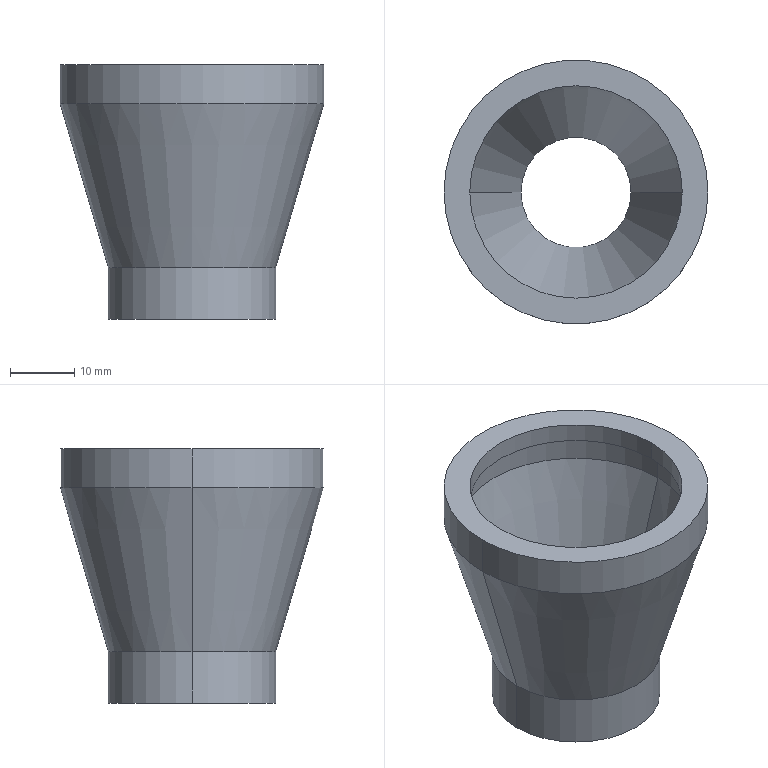Part | NX | features BREP 1 | 1 solid | 15 faces | box 41 x 41 x 39.5 mm | volume 9433 mm3 | cylinder 8 | cone 4 | plane 3 | commonest cylinder face diameters 26 x2 33 x2 36 x2 41 x2
STEP:
#1=CARTESIAN_POINT('',(13.,0.,-51.5));
#2=VERTEX_POINT('',#1);
#3=CARTESIAN_POINT('',(-13.,0.,-51.5));
#4=VERTEX_POINT('',#3);
#5=CARTESIAN_POINT('',(0.,0.,-51.5));
#6=DIRECTION('',(0.,0.,1.));
#7=DIRECTION('',(1.,0.,0.));
#8=AXIS2_PLACEMENT_3D('',#5,#6,#7);
#9=CIRCLE('',#8,13.);
#10=EDGE_CURVE('',#2,#4,#9,.T.);
#11=ORIENTED_EDGE('',*,*,#10,.T.);
#12=CARTESIAN_POINT('',(-20.5,0.,-26.));
#13=VERTEX_POINT('',#12);
#14=CARTESIAN_POINT('',(-20.5,0.,-26.));
#15=DIRECTION('',(-0.2822,0.,0.9594));
#16=VECTOR('',#15,1000.);
#17=LINE('',#14,#16);
#18=EDGE_CURVE('',#13,#4,#17,.F.);
#19=ORIENTED_EDGE('',*,*,#18,.F.);
#20=CARTESIAN_POINT('',(20.5,0.,-26.));
#21=VERTEX_POINT('',#20);
#22=CARTESIAN_POINT('',(0.,0.,-26.));
#23=DIRECTION('',(0.,0.,-1.));
#24=DIRECTION('',(1.,0.,0.));
#25=AXIS2_PLACEMENT_3D('',#22,#23,#24);
#26=CIRCLE('',#25,20.5);
#27=EDGE_CURVE('',#13,#21,#26,.T.);
#28=ORIENTED_EDGE('',*,*,#27,.T.);
#29=CARTESIAN_POINT('',(20.5,0.,-26.));
#30=DIRECTION('',(0.2822,0.,0.9594));
#31=VECTOR('',#30,1000.);
#32=LINE('',#29,#31);
#33=EDGE_CURVE('',#21,#2,#32,.F.);
#34=ORIENTED_EDGE('',*,*,#33,.T.);
#35=EDGE_LOOP('',(#11,#19,#28,#34));
#36=FACE_BOUND('',#35,.T.);
#37=CARTESIAN_POINT('',(0.,0.,-26.));
#38=DIRECTION('',(0.,0.,1.));
#39=DIRECTION('',(1.,0.,0.));
#40=AXIS2_PLACEMENT_3D('',#37,#38,#39);
#41=CONICAL_SURFACE('',#40,20.5,0.2861);
#42=ADVANCED_FACE('',(#36),#41,.T.);
#43=CARTESIAN_POINT('',(-20.5,0.,-20.));
#44=VERTEX_POINT('',#43);
#45=CARTESIAN_POINT('',(20.5,0.,-20.));
#46=VERTEX_POINT('',#45);
#47=CARTESIAN_POINT('',(0.,0.,-20.));
#48=DIRECTION('',(0.,0.,-1.));
#49=DIRECTION('',(-1.,0.,0.));
#50=AXIS2_PLACEMENT_3D('',#47,#48,#49);
#51=CIRCLE('',#50,20.5);
#52=EDGE_CURVE('',#44,#46,#51,.T.);
#53=ORIENTED_EDGE('',*,*,#52,.T.);
#54=CARTESIAN_POINT('',(20.5,0.,-23.));
#55=DIRECTION('',(0.,0.,-1.));
#56=VECTOR('',#55,1000.);
#57=LINE('',#54,#56);
#58=EDGE_CURVE('',#46,#21,#57,.T.);
#59=ORIENTED_EDGE('',*,*,#58,.T.);
#60=ORIENTED_EDGE('',*,*,#27,.F.);
#61=CARTESIAN_POINT('',(-20.5,0.,-23.));
#62=DIRECTION('',(0.,0.,-1.));
#63=VECTOR('',#62,1000.);
#64=LINE('',#61,#63);
#65=EDGE_CURVE('',#44,#13,#64,.T.);
#66=ORIENTED_EDGE('',*,*,#65,.F.);
#67=EDGE_LOOP('',(#53,#59,#60,#66));
#68=FACE_BOUND('',#67,.T.);
#69=CARTESIAN_POINT('',(0.,0.,-23.));
#70=DIRECTION('',(0.,0.,-1.));
#71=DIRECTION('',(-1.,0.,0.));
#72=AXIS2_PLACEMENT_3D('',#69,#70,#71);
#73=CYLINDRICAL_SURFACE('',#72,20.5);
#74=ADVANCED_FACE('',(#68),#73,.T.);
#75=ORIENTED_EDGE('',*,*,#10,.F.);
#76=CARTESIAN_POINT('',(13.,0.,-59.5));
#77=VERTEX_POINT('',#76);
#78=CARTESIAN_POINT('',(13.,0.,-55.5));
#79=DIRECTION('',(0.,0.,-1.));
#80=VECTOR('',#79,1000.);
#81=LINE('',#78,#80);
#82=EDGE_CURVE('',#2,#77,#81,.T.);
#83=ORIENTED_EDGE('',*,*,#82,.T.);
#84=CARTESIAN_POINT('',(-13.,0.,-59.5));
#85=VERTEX_POINT('',#84);
#86=CARTESIAN_POINT('',(0.,0.,-59.5));
#87=DIRECTION('',(0.,0.,1.));
#88=DIRECTION('',(-1.,0.,0.));
#89=AXIS2_PLACEMENT_3D('',#86,#87,#88);
#90=CIRCLE('',#89,13.);
#91=EDGE_CURVE('',#77,#85,#90,.T.);
#92=ORIENTED_EDGE('',*,*,#91,.T.);
#93=CARTESIAN_POINT('',(-13.,0.,-55.5));
#94=DIRECTION('',(0.,0.,-1.));
#95=VECTOR('',#94,1000.);
#96=LINE('',#93,#95);
#97=EDGE_CURVE('',#4,#85,#96,.T.);
#98=ORIENTED_EDGE('',*,*,#97,.F.);
#99=EDGE_LOOP('',(#75,#83,#92,#98));
#100=FACE_BOUND('',#99,.T.);
#101=CARTESIAN_POINT('',(0.,0.,-55.5));
#102=DIRECTION('',(0.,0.,-1.));
#103=DIRECTION('',(-1.,0.,0.));
#104=AXIS2_PLACEMENT_3D('',#101,#102,#103);
#105=CYLINDRICAL_SURFACE('',#104,13.);
#106=ADVANCED_FACE('',(#100),#105,.T.);
#107=CARTESIAN_POINT('',(16.5,0.,-20.));
#108=VERTEX_POINT('',#107);
#109=CARTESIAN_POINT('',(-16.5,0.,-20.));
#110=VERTEX_POINT('',#109);
#111=CARTESIAN_POINT('',(0.,0.,-20.));
#112=DIRECTION('',(0.,0.,-1.));
#113=DIRECTION('',(-1.,0.,0.));
#114=AXIS2_PLACEMENT_3D('',#111,#112,#113);
#115=CIRCLE('',#114,16.5);
#116=EDGE_CURVE('',#108,#110,#115,.T.);
#117=ORIENTED_EDGE('',*,*,#116,.F.);
#118=CARTESIAN_POINT('',(16.5,0.,-22.99));
#119=VERTEX_POINT('',#118);
#120=CARTESIAN_POINT('',(16.5,0.,-21.495));
#121=DIRECTION('',(0.,0.,-1.));
#122=VECTOR('',#121,1000.);
#123=LINE('',#120,#122);
#124=EDGE_CURVE('',#108,#119,#123,.T.);
#125=ORIENTED_EDGE('',*,*,#124,.T.);
#126=CARTESIAN_POINT('',(-16.5,0.,-22.99));
#127=VERTEX_POINT('',#126);
#128=CARTESIAN_POINT('',(0.,0.,-22.99));
#129=DIRECTION('',(0.,0.,1.));
#130=DIRECTION('',(-1.,0.,0.));
#131=AXIS2_PLACEMENT_3D('',#128,#129,#130);
#132=CIRCLE('',#131,16.5);
#133=EDGE_CURVE('',#127,#119,#132,.T.);
#134=ORIENTED_EDGE('',*,*,#133,.F.);
#135=CARTESIAN_POINT('',(-16.5,0.,-21.495));
#136=DIRECTION('',(0.,0.,-1.));
#137=VECTOR('',#136,1000.);
#138=LINE('',#135,#137);
#139=EDGE_CURVE('',#110,#127,#138,.T.);
#140=ORIENTED_EDGE('',*,*,#139,.F.);
#141=EDGE_LOOP('',(#117,#125,#134,#140));
#142=FACE_BOUND('',#141,.T.);
#143=CARTESIAN_POINT('',(0.,0.,-21.495));
#144=DIRECTION('',(0.,0.,-1.));
#145=DIRECTION('',(-1.,0.,0.));
#146=AXIS2_PLACEMENT_3D('',#143,#144,#145);
#147=CYLINDRICAL_SURFACE('',#146,16.5);
#148=ADVANCED_FACE('',(#142),#147,.F.);
#149=CARTESIAN_POINT('',(-8.562,0.,-59.5));
#150=VERTEX_POINT('',#149);
#151=CARTESIAN_POINT('',(8.562,0.,-59.5));
#152=VERTEX_POINT('',#151);
#153=CARTESIAN_POINT('',(0.,0.,-59.5));
#154=DIRECTION('',(0.,0.,1.));
#155=DIRECTION('',(1.,0.,0.));
#156=AXIS2_PLACEMENT_3D('',#153,#154,#155);
#157=CIRCLE('',#156,8.562);
#158=EDGE_CURVE('',#150,#152,#157,.T.);
#159=ORIENTED_EDGE('',*,*,#158,.F.);
#160=CARTESIAN_POINT('',(-18.,0.,-27.412));
#161=VERTEX_POINT('',#160);
#162=CARTESIAN_POINT('',(-18.,0.,-27.412));
#163=DIRECTION('',(-0.2822,0.,0.9594));
#164=VECTOR('',#163,1000.);
#165=LINE('',#162,#164);
#166=EDGE_CURVE('',#161,#150,#165,.F.);
#167=ORIENTED_EDGE('',*,*,#166,.F.);
#168=CARTESIAN_POINT('',(18.,0.,-27.412));
#169=VERTEX_POINT('',#168);
#170=CARTESIAN_POINT('',(0.,0.,-27.412));
#171=DIRECTION('',(0.,0.,-1.));
#172=DIRECTION('',(1.,0.,0.));
#173=AXIS2_PLACEMENT_3D('',#170,#171,#172);
#174=CIRCLE('',#173,18.);
#175=EDGE_CURVE('',#169,#161,#174,.T.);
#176=ORIENTED_EDGE('',*,*,#175,.F.);
#177=CARTESIAN_POINT('',(18.,0.,-27.412));
#178=DIRECTION('',(0.2822,0.,0.9594));
#179=VECTOR('',#178,1000.);
#180=LINE('',#177,#179);
#181=EDGE_CURVE('',#169,#152,#180,.F.);
#182=ORIENTED_EDGE('',*,*,#181,.T.);
#183=EDGE_LOOP('',(#159,#167,#176,#182));
#184=FACE_BOUND('',#183,.T.);
#185=CARTESIAN_POINT('',(0.,0.,-27.412));
#186=DIRECTION('',(0.,0.,1.));
#187=DIRECTION('',(1.,0.,0.));
#188=AXIS2_PLACEMENT_3D('',#185,#186,#187);
#189=CONICAL_SURFACE('',#188,18.,0.2861);
#190=ADVANCED_FACE('',(#184),#189,.F.);
#191=CARTESIAN_POINT('',(18.,0.,-22.99));
#192=VERTEX_POINT('',#191);
#193=CARTESIAN_POINT('',(-18.,0.,-22.99));
#194=VERTEX_POINT('',#193);
#195=CARTESIAN_POINT('',(0.,0.,-22.99));
#196=DIRECTION('',(0.,0.,-1.));
#197=DIRECTION('',(-1.,0.,0.));
#198=AXIS2_PLACEMENT_3D('',#195,#196,#197);
#199=CIRCLE('',#198,18.);
#200=EDGE_CURVE('',#192,#194,#199,.T.);
#201=ORIENTED_EDGE('',*,*,#200,.F.);
#202=CARTESIAN_POINT('',(18.,0.,-25.201));
#203=DIRECTION('',(0.,0.,-1.));
#204=VECTOR('',#203,1000.);
#205=LINE('',#202,#204);
#206=EDGE_CURVE('',#192,#169,#205,.T.);
#207=ORIENTED_EDGE('',*,*,#206,.T.);
#208=ORIENTED_EDGE('',*,*,#175,.T.);
#209=CARTESIAN_POINT('',(-18.,0.,-25.201));
#210=DIRECTION('',(0.,0.,-1.));
#211=VECTOR('',#210,1000.);
#212=LINE('',#209,#211);
#213=EDGE_CURVE('',#194,#161,#212,.T.);
#214=ORIENTED_EDGE('',*,*,#213,.F.);
#215=EDGE_LOOP('',(#201,#207,#208,#214));
#216=FACE_BOUND('',#215,.T.);
#217=CARTESIAN_POINT('',(0.,0.,-25.201));
#218=DIRECTION('',(0.,0.,-1.));
#219=DIRECTION('',(-1.,0.,0.));
#220=AXIS2_PLACEMENT_3D('',#217,#218,#219);
#221=CYLINDRICAL_SURFACE('',#220,18.);
#222=ADVANCED_FACE('',(#216),#221,.F.);
#223=ORIENTED_EDGE('',*,*,#18,.T.);
#224=CARTESIAN_POINT('',(0.,0.,-51.5));
#225=DIRECTION('',(0.,0.,1.));
#226=DIRECTION('',(1.,0.,0.));
#227=AXIS2_PLACEMENT_3D('',#224,#225,#226);
#228=CIRCLE('',#227,13.);
#229=EDGE_CURVE('',#4,#2,#228,.T.);
#230=ORIENTED_EDGE('',*,*,#229,.T.);
#231=ORIENTED_EDGE('',*,*,#33,.F.);
#232=CARTESIAN_POINT('',(0.,0.,-26.));
#233=DIRECTION('',(0.,0.,-1.));
#234=DIRECTION('',(1.,0.,0.));
#235=AXIS2_PLACEMENT_3D('',#232,#233,#234);
#236=CIRCLE('',#235,20.5);
#237=EDGE_CURVE('',#21,#13,#236,.T.);
#238=ORIENTED_EDGE('',*,*,#237,.T.);
#239=EDGE_LOOP('',(#223,#230,#231,#238));
#240=FACE_BOUND('',#239,.T.);
#241=CARTESIAN_POINT('',(0.,0.,-26.));
#242=DIRECTION('',(0.,0.,1.));
#243=DIRECTION('',(1.,0.,0.));
#244=AXIS2_PLACEMENT_3D('',#241,#242,#243);
#245=CONICAL_SURFACE('',#244,20.5,0.2861);
#246=ADVANCED_FACE('',(#240),#245,.T.);
#247=ORIENTED_EDGE('',*,*,#58,.F.);
#248=CARTESIAN_POINT('',(0.,0.,-20.));
#249=DIRECTION('',(0.,0.,-1.));
#250=DIRECTION('',(-1.,0.,0.));
#251=AXIS2_PLACEMENT_3D('',#248,#249,#250);
#252=CIRCLE('',#251,20.5);
#253=EDGE_CURVE('',#46,#44,#252,.T.);
#254=ORIENTED_EDGE('',*,*,#253,.T.);
#255=ORIENTED_EDGE('',*,*,#65,.T.);
#256=ORIENTED_EDGE('',*,*,#237,.F.);
#257=EDGE_LOOP('',(#247,#254,#255,#256));
#258=FACE_BOUND('',#257,.T.);
#259=CARTESIAN_POINT('',(0.,0.,-23.));
#260=DIRECTION('',(0.,0.,-1.));
#261=DIRECTION('',(-1.,0.,0.));
#262=AXIS2_PLACEMENT_3D('',#259,#260,#261);
#263=CYLINDRICAL_SURFACE('',#262,20.5);
#264=ADVANCED_FACE('',(#258),#263,.T.);
#265=ORIENTED_EDGE('',*,*,#82,.F.);
#266=ORIENTED_EDGE('',*,*,#229,.F.);
#267=ORIENTED_EDGE('',*,*,#97,.T.);
#268=CARTESIAN_POINT('',(0.,0.,-59.5));
#269=DIRECTION('',(0.,0.,1.));
#270=DIRECTION('',(-1.,0.,0.));
#271=AXIS2_PLACEMENT_3D('',#268,#269,#270);
#272=CIRCLE('',#271,13.);
#273=EDGE_CURVE('',#85,#77,#272,.T.);
#274=ORIENTED_EDGE('',*,*,#273,.T.);
#275=EDGE_LOOP('',(#265,#266,#267,#274));
#276=FACE_BOUND('',#275,.T.);
#277=CARTESIAN_POINT('',(0.,0.,-55.5));
#278=DIRECTION('',(0.,0.,-1.));
#279=DIRECTION('',(-1.,0.,0.));
#280=AXIS2_PLACEMENT_3D('',#277,#278,#279);
#281=CYLINDRICAL_SURFACE('',#280,13.);
#282=ADVANCED_FACE('',(#276),#281,.T.);
#283=ORIENTED_EDGE('',*,*,#52,.F.);
#284=ORIENTED_EDGE('',*,*,#253,.F.);
#285=EDGE_LOOP('',(#283,#284));
#286=FACE_BOUND('',#285,.T.);
#287=CARTESIAN_POINT('',(0.,0.,-20.));
#288=DIRECTION('',(0.,0.,-1.));
#289=DIRECTION('',(-1.,0.,0.));
#290=AXIS2_PLACEMENT_3D('',#287,#288,#289);
#291=CIRCLE('',#290,16.5);
#292=EDGE_CURVE('',#110,#108,#291,.T.);
#293=ORIENTED_EDGE('',*,*,#292,.T.);
#294=ORIENTED_EDGE('',*,*,#116,.T.);
#295=EDGE_LOOP('',(#293,#294));
#296=FACE_BOUND('',#295,.T.);
#297=CARTESIAN_POINT('',(0.,18.5,-20.));
#298=DIRECTION('',(0.,0.,1.));
#299=DIRECTION('',(1.,0.,0.));
#300=AXIS2_PLACEMENT_3D('',#297,#298,#299);
#301=PLANE('',#300);
#302=ADVANCED_FACE('',(#286,#296),#301,.T.);
#303=ORIENTED_EDGE('',*,*,#273,.F.);
#304=ORIENTED_EDGE('',*,*,#91,.F.);
#305=EDGE_LOOP('',(#303,#304));
#306=FACE_BOUND('',#305,.T.);
#307=CARTESIAN_POINT('',(0.,0.,-59.5));
#308=DIRECTION('',(0.,0.,1.));
#309=DIRECTION('',(1.,0.,0.));
#310=AXIS2_PLACEMENT_3D('',#307,#308,#309);
#311=CIRCLE('',#310,8.562);
#312=EDGE_CURVE('',#152,#150,#311,.T.);
#313=ORIENTED_EDGE('',*,*,#312,.T.);
#314=ORIENTED_EDGE('',*,*,#158,.T.);
#315=EDGE_LOOP('',(#313,#314));
#316=FACE_BOUND('',#315,.T.);
#317=CARTESIAN_POINT('',(0.,10.781,-59.5));
#318=DIRECTION('',(0.,0.,-1.));
#319=DIRECTION('',(0.,-1.,0.));
#320=AXIS2_PLACEMENT_3D('',#317,#318,#319);
#321=PLANE('',#320);
#322=ADVANCED_FACE('',(#306,#316),#321,.T.);
#323=ORIENTED_EDGE('',*,*,#124,.F.);
#324=ORIENTED_EDGE('',*,*,#292,.F.);
#325=ORIENTED_EDGE('',*,*,#139,.T.);
#326=CARTESIAN_POINT('',(0.,0.,-22.99));
#327=DIRECTION('',(0.,0.,1.));
#328=DIRECTION('',(-1.,0.,0.));
#329=AXIS2_PLACEMENT_3D('',#326,#327,#328);
#330=CIRCLE('',#329,16.5);
#331=EDGE_CURVE('',#119,#127,#330,.T.);
#332=ORIENTED_EDGE('',*,*,#331,.F.);
#333=EDGE_LOOP('',(#323,#324,#325,#332));
#334=FACE_BOUND('',#333,.T.);
#335=CARTESIAN_POINT('',(0.,0.,-21.495));
#336=DIRECTION('',(0.,0.,-1.));
#337=DIRECTION('',(-1.,0.,0.));
#338=AXIS2_PLACEMENT_3D('',#335,#336,#337);
#339=CYLINDRICAL_SURFACE('',#338,16.5);
#340=ADVANCED_FACE('',(#334),#339,.F.);
#341=ORIENTED_EDGE('',*,*,#166,.T.);
#342=ORIENTED_EDGE('',*,*,#312,.F.);
#343=ORIENTED_EDGE('',*,*,#181,.F.);
#344=CARTESIAN_POINT('',(0.,0.,-27.412));
#345=DIRECTION('',(0.,0.,-1.));
#346=DIRECTION('',(1.,0.,0.));
#347=AXIS2_PLACEMENT_3D('',#344,#345,#346);
#348=CIRCLE('',#347,18.);
#349=EDGE_CURVE('',#161,#169,#348,.T.);
#350=ORIENTED_EDGE('',*,*,#349,.F.);
#351=EDGE_LOOP('',(#341,#342,#343,#350));
#352=FACE_BOUND('',#351,.T.);
#353=CARTESIAN_POINT('',(0.,0.,-27.412));
#354=DIRECTION('',(0.,0.,1.));
#355=DIRECTION('',(1.,0.,0.));
#356=AXIS2_PLACEMENT_3D('',#353,#354,#355);
#357=CONICAL_SURFACE('',#356,18.,0.2861);
#358=ADVANCED_FACE('',(#352),#357,.F.);
#359=CARTESIAN_POINT('',(0.,0.,-22.99));
#360=DIRECTION('',(0.,0.,-1.));
#361=DIRECTION('',(-1.,0.,0.));
#362=AXIS2_PLACEMENT_3D('',#359,#360,#361);
#363=CIRCLE('',#362,18.);
#364=EDGE_CURVE('',#194,#192,#363,.T.);
#365=ORIENTED_EDGE('',*,*,#364,.T.);
#366=ORIENTED_EDGE('',*,*,#200,.T.);
#367=EDGE_LOOP('',(#365,#366));
#368=FACE_BOUND('',#367,.T.);
#369=ORIENTED_EDGE('',*,*,#133,.T.);
#370=ORIENTED_EDGE('',*,*,#331,.T.);
#371=EDGE_LOOP('',(#369,#370));
#372=FACE_BOUND('',#371,.T.);
#373=CARTESIAN_POINT('',(0.,17.25,-22.99));
#374=DIRECTION('',(0.,0.,-1.));
#375=DIRECTION('',(0.,-1.,0.));
#376=AXIS2_PLACEMENT_3D('',#373,#374,#375);
#377=PLANE('',#376);
#378=ADVANCED_FACE('',(#368,#372),#377,.T.);
#379=ORIENTED_EDGE('',*,*,#206,.F.);
#380=ORIENTED_EDGE('',*,*,#364,.F.);
#381=ORIENTED_EDGE('',*,*,#213,.T.);
#382=ORIENTED_EDGE('',*,*,#349,.T.);
#383=EDGE_LOOP('',(#379,#380,#381,#382));
#384=FACE_BOUND('',#383,.T.);
#385=CARTESIAN_POINT('',(0.,0.,-25.201));
#386=DIRECTION('',(0.,0.,-1.));
#387=DIRECTION('',(-1.,0.,0.));
#388=AXIS2_PLACEMENT_3D('',#385,#386,#387);
#389=CYLINDRICAL_SURFACE('',#388,18.);
#390=ADVANCED_FACE('',(#384),#389,.F.);
#391=CLOSED_SHELL('',(#42,#74,#106,#148,#190,#222,#246,#264,#282,#302,#322,#340,#358,#378,#390));
#392=MANIFOLD_SOLID_BREP('',#391);
#393=(LENGTH_UNIT()NAMED_UNIT(*)SI_UNIT(.MILLI.,.METRE.));
#394=UNCERTAINTY_MEASURE_WITH_UNIT(LENGTH_MEASURE(0.00001),#393,'','');
#395=(NAMED_UNIT(*)PLANE_ANGLE_UNIT()SI_UNIT($,.RADIAN.));
#396=(NAMED_UNIT(*)SI_UNIT($,.STERADIAN.)SOLID_ANGLE_UNIT());
#397=(GEOMETRIC_REPRESENTATION_CONTEXT(3)GLOBAL_UNCERTAINTY_ASSIGNED_CONTEXT((#394))GLOBAL_UNIT_ASSIGNED_CONTEXT((#393,#395,#396))REPRESENTATION_CONTEXT('',''));
#398=ADVANCED_BREP_SHAPE_REPRESENTATION('',(#392),#397);